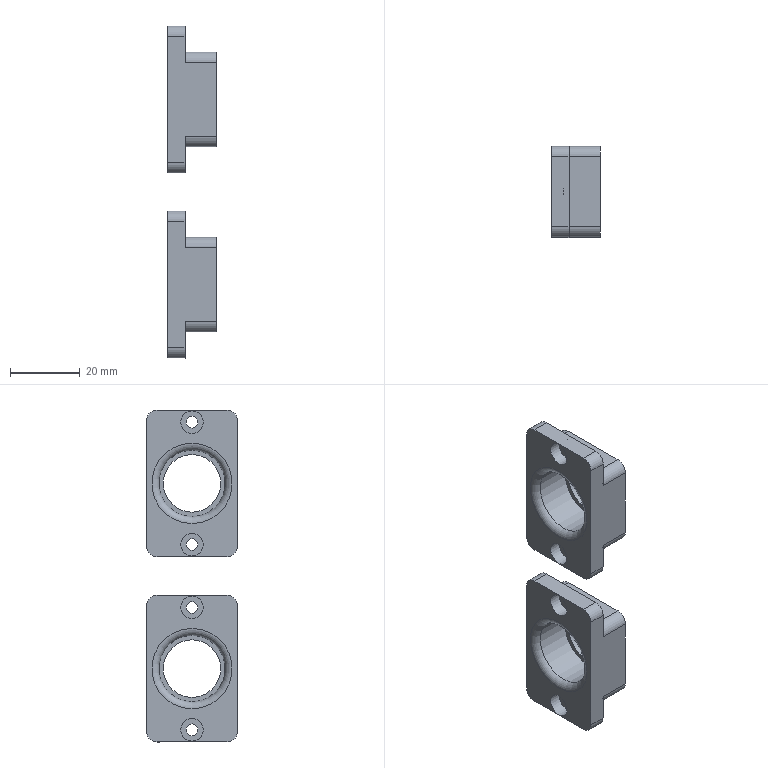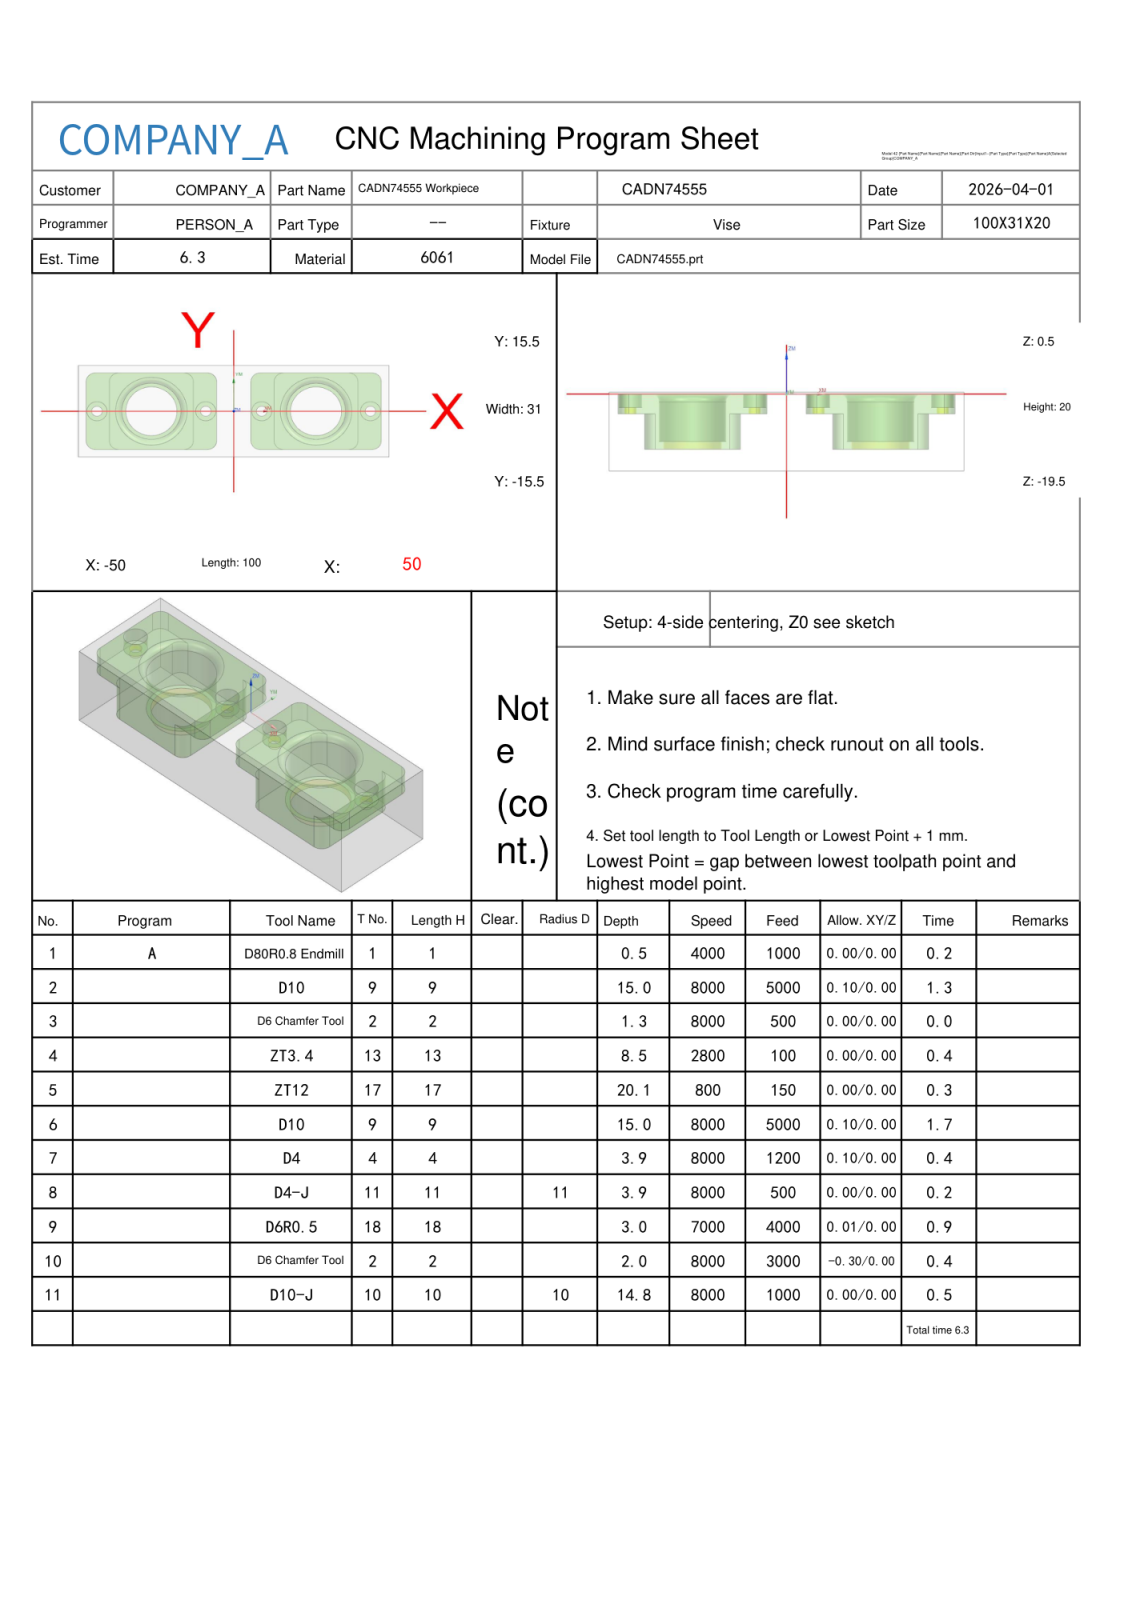NC program | NX | posted by the shop | part box 14 x 26 x 95 mm
Lines 1 to 426 of 19918:
%
O0001
(Machine time: 8.47 MIN)
(===Total Tool:9===)
(T1=D80R0.8 Endmill D=80.  R=0.8  D-  H01 Z=-0.   )
(T9=D10     D=10.  R=0.   D-  H09 Z=-14.5 )
(T2=D6 Chamfer tool   D=6.   R=0.   D-  H02 Z=-1.5  )
(T13=ZT3.4  D=3.4  DR_a=118 D-  H13 Z=-8.02 )
(T17=ZT12   D=12.  DR_a=118 D-  H17 Z=-19.61)
(T4=D4      D=4.   R=0.   D-  H04 Z=-3.4  )
(T11=D4-J   D=4.   R=0.   D11 H11 Z=-3.4  )
(T18=D6R0.5 D=6.   R=0.5  D-  H18 Z=-2.5  )
(T10=D10-J  D=10.  R=0.   D10 H10 Z=-14.3 )
G80 G90 G17 G49 G40
G91 G28 Z0
M01
N1 T01 M06
(D80R0.8 Endmill  D=80. R=0.8 H=01 ce=0.00 di=0.00)
G00 G90 G54 X92.5 Y0.0 M03 S4000
G43 H01 Z20.
M08
Z2.
G01 Z0.0 F1000.
X87.5
X-87.5
X-92.5
Z2.
G00 Z20.
G91 G28 Z0.0
M05
M09
G91 G28 Z0.0
M01
N2 T09 M06
(D10  D=10. R=0. H=09 ce=0.10 di=0.00)
G00 G90 G54 X-26.5 Y18.1 M03 S8000
G43 H09 Z20.
M08
Z.5
G01 X-8.5 Z.413 F5000.
G02 X-.4 Y10. Z.351 I0.0 J-8.1
G01 Y-10. Z.254
G02 X-8.5 Y-18.1 Z.193 I-8.1 J0.0
G01 X-44.5 Z.018
G02 X-52.6 Y-10. Z-.044 I0.0 J8.1
G01 Y10. Z-.141
G02 X-44.5 Y18.1 Z-.202 I8.1 J0.0
G01 X-8.5 Z-.377
G02 X-.4 Y10. Z-.438 I0.0 J-8.1
G01 Y-10. Z-.535
G02 X-8.5 Y-18.1 Z-.597 I-8.1 J0.0
G01 X-44.5 Z-.771
G02 X-52.6 Y-10. Z-.833 I0.0 J8.1
G01 Y10. Z-.93
G02 X-44.5 Y18.1 Z-.992 I8.1 J0.0
G01 X-8.5 Z-1.166
G02 X-.4 Y10. Z-1.228 I0.0 J-8.1
G01 Y-10. Z-1.325
G02 X-8.5 Y-18.1 Z-1.386 I-8.1 J0.0
G01 X-44.5 Z-1.561
G02 X-52.6 Y-10. Z-1.623 I0.0 J8.1
G01 Y10. Z-1.72
G02 X-44.5 Y18.1 Z-1.781 I8.1 J0.0
G01 X-8.5 Z-1.956
G02 X-.4 Y10. Z-2.017 I0.0 J-8.1
G01 Y-10. Z-2.114
G02 X-8.5 Y-18.1 Z-2.176 I-8.1 J0.0
G01 X-44.5 Z-2.35
G02 X-52.6 Y-10. Z-2.412 I0.0 J8.1
G01 Y10. Z-2.509
G02 X-44.5 Y18.1 Z-2.571 I8.1 J0.0
G01 X-8.5 Z-2.745
G02 X-.4 Y10. Z-2.807 I0.0 J-8.1
G01 Y-10. Z-2.904
G02 X-8.5 Y-18.1 Z-2.965 I-8.1 J0.0
G01 X-44.5 Z-3.14
G02 X-52.6 Y-10. Z-3.202 I0.0 J8.1
G01 Y10. Z-3.298
G02 X-44.5 Y18.1 Z-3.36 I8.1 J0.0
G01 X-8.5 Z-3.535
G02 X-.4 Y10. Z-3.596 I0.0 J-8.1
G01 Y-10. Z-3.693
G02 X-8.5 Y-18.1 Z-3.755 I-8.1 J0.0
G01 X-44.5 Z-3.929
G02 X-52.6 Y-10. Z-3.991 I0.0 J8.1
G01 Y10. Z-4.088
G02 X-44.5 Y18.1 Z-4.15 I8.1 J0.0
G01 X-8.5 Z-4.324
G02 X-.4 Y10. Z-4.386 I0.0 J-8.1
G01 Y-10. Z-4.483
G02 X-8.5 Y-18.1 Z-4.544 I-8.1 J0.0
G01 X-44.5 Z-4.719
G02 X-52.6 Y-10. Z-4.78 I0.0 J8.1
G01 Y10. Z-4.877
G02 X-44.5 Y18.1 Z-4.939 I8.1 J0.0
G01 X-8.5 Z-5.114
G02 X-.4 Y10. Z-5.175 I0.0 J-8.1
G01 Y-10. Z-5.272
G02 X-8.5 Y-18.1 Z-5.334 I-8.1 J0.0
G01 X-44.5 Z-5.508
G02 X-52.6 Y-10. Z-5.57 I0.0 J8.1
G01 Y10. Z-5.667
G02 X-44.5 Y18.1 Z-5.729 I8.1 J0.0
G01 X-8.5 Z-5.903
G02 X-.4 Y10. Z-5.965 I0.0 J-8.1
G01 Y-10. Z-6.062
G02 X-8.5 Y-18.1 Z-6.123 I-8.1 J0.0
G01 X-44.5 Z-6.298
G02 X-52.6 Y-10. Z-6.359 I0.0 J8.1
G01 Y10. Z-6.456
G02 X-44.5 Y18.1 Z-6.518 I8.1 J0.0
G01 X-8.5 Z-6.693
G02 X-.4 Y10. Z-6.754 I0.0 J-8.1
G01 Y-10. Z-6.851
G02 X-8.5 Y-18.1 Z-6.913 I-8.1 J0.0
G01 X-44.5 Z-7.087
G02 X-52.6 Y-10. Z-7.149 I0.0 J8.1
G01 Y10. Z-7.246
G02 X-44.5 Y18.1 Z-7.307 I8.1 J0.0
G01 X-8.5 Z-7.482
G02 X-.4 Y10. Z-7.544 I0.0 J-8.1
G01 Y-10. Z-7.641
G02 X-8.5 Y-18.1 Z-7.702 I-8.1 J0.0
G01 X-44.5 Z-7.877
G02 X-52.6 Y-10. Z-7.938 I0.0 J8.1
G01 Y10. Z-8.035
G02 X-44.5 Y18.1 Z-8.097 I8.1 J0.0
G01 X-8.5 Z-8.271
G02 X-.4 Y10. Z-8.333 I0.0 J-8.1
G01 Y-10. Z-8.43
G02 X-8.5 Y-18.1 Z-8.492 I-8.1 J0.0
G01 X-44.5 Z-8.666
G02 X-52.6 Y-10. Z-8.728 I0.0 J8.1
G01 Y10. Z-8.825
G02 X-44.5 Y18.1 Z-8.886 I8.1 J0.0
G01 X-8.5 Z-9.061
G02 X-.4 Y10. Z-9.123 I0.0 J-8.1
G01 Y-10. Z-9.22
G02 X-8.5 Y-18.1 Z-9.281 I-8.1 J0.0
G01 X-44.5 Z-9.456
G02 X-52.6 Y-10. Z-9.517 I0.0 J8.1
G01 Y10. Z-9.614
G02 X-44.5 Y18.1 Z-9.676 I8.1 J0.0
G01 X-8.5 Z-9.85
G02 X-.4 Y10. Z-9.912 I0.0 J-8.1
G01 Y-10. Z-10.009
G02 X-8.5 Y-18.1 Z-10.071 I-8.1 J0.0
G01 X-44.5 Z-10.245
G02 X-52.6 Y-10. Z-10.307 I0.0 J8.1
G01 Y10. Z-10.404
G02 X-44.5 Y18.1 Z-10.465 I8.1 J0.0
G01 X-8.5 Z-10.64
G02 X-.4 Y10. Z-10.702 I0.0 J-8.1
G01 Y-10. Z-10.798
G02 X-8.5 Y-18.1 Z-10.86 I-8.1 J0.0
G01 X-44.5 Z-11.035
G02 X-52.6 Y-10. Z-11.096 I0.0 J8.1
G01 Y10. Z-11.193
G02 X-44.5 Y18.1 Z-11.255 I8.1 J0.0
G01 X-8.5 Z-11.429
G02 X-.4 Y10. Z-11.491 I0.0 J-8.1
G01 Y-10. Z-11.588
G02 X-8.5 Y-18.1 Z-11.65 I-8.1 J0.0
G01 X-44.5 Z-11.824
G02 X-52.6 Y-10. Z-11.886 I0.0 J8.1
G01 Y10. Z-11.983
G02 X-44.5 Y18.1 Z-12.044 I8.1 J0.0
G01 X-8.5 Z-12.219
G02 X-.4 Y10. Z-12.28 I0.0 J-8.1
G01 Y-10. Z-12.377
G02 X-8.5 Y-18.1 Z-12.439 I-8.1 J0.0
G01 X-44.5 Z-12.614
G02 X-52.6 Y-10. Z-12.675 I0.0 J8.1
G01 Y10. Z-12.772
G02 X-44.5 Y18.1 Z-12.834 I8.1 J0.0
G01 X-8.5 Z-13.008
G02 X-.4 Y10. Z-13.07 I0.0 J-8.1
G01 Y-10. Z-13.167
G02 X-8.5 Y-18.1 Z-13.229 I-8.1 J0.0
G01 X-44.5 Z-13.403
G02 X-52.6 Y-10. Z-13.465 I0.0 J8.1
G01 Y10. Z-13.562
G02 X-44.5 Y18.1 Z-13.623 I8.1 J0.0
G01 X-8.5 Z-13.798
G02 X-.4 Y10. Z-13.859 I0.0 J-8.1
G01 Y-10. Z-13.956
G02 X-8.5 Y-18.1 Z-14.018 I-8.1 J0.0
G01 X-44.5 Z-14.193
G02 X-52.6 Y-10. Z-14.254 I0.0 J8.1
G01 Y10. Z-14.351
G02 X-44.5 Y18.1 Z-14.413 I8.1 J0.0
G01 X-26.5 Z-14.5
X-8.5
G02 X-.4 Y10. I0.0 J-8.1
G01 Y-10.
G02 X-8.5 Y-18.1 I-8.1 J0.0
G01 X-44.5
G02 X-52.6 Y-10. I0.0 J8.1
G01 Y10.
G02 X-44.5 Y18.1 I8.1 J0.0
G01 X-26.5
X-26.
Z-13.5
G00 Z20.
X26.5
Z.5
G01 X44.5 Z.413
G02 X52.6 Y10. Z.351 I0.0 J-8.1
G01 Y-10. Z.254
G02 X44.5 Y-18.1 Z.193 I-8.1 J0.0
G01 X8.5 Z.018
G02 X.4 Y-10. Z-.044 I0.0 J8.1
G01 Y10. Z-.141
G02 X8.5 Y18.1 Z-.202 I8.1 J0.0
G01 X44.5 Z-.377
G02 X52.6 Y10. Z-.438 I0.0 J-8.1
G01 Y-10. Z-.535
G02 X44.5 Y-18.1 Z-.597 I-8.1 J0.0
G01 X8.5 Z-.771
G02 X.4 Y-10. Z-.833 I0.0 J8.1
G01 Y10. Z-.93
G02 X8.5 Y18.1 Z-.992 I8.1 J0.0
G01 X44.5 Z-1.166
G02 X52.6 Y10. Z-1.228 I0.0 J-8.1
G01 Y-10. Z-1.325
G02 X44.5 Y-18.1 Z-1.386 I-8.1 J0.0
G01 X8.5 Z-1.561
G02 X.4 Y-10. Z-1.623 I0.0 J8.1
G01 Y10. Z-1.72
G02 X8.5 Y18.1 Z-1.781 I8.1 J0.0
G01 X44.5 Z-1.956
G02 X52.6 Y10. Z-2.017 I0.0 J-8.1
G01 Y-10. Z-2.114
G02 X44.5 Y-18.1 Z-2.176 I-8.1 J0.0
G01 X8.5 Z-2.35
G02 X.4 Y-10. Z-2.412 I0.0 J8.1
G01 Y10. Z-2.509
G02 X8.5 Y18.1 Z-2.571 I8.1 J0.0
G01 X44.5 Z-2.745
G02 X52.6 Y10. Z-2.807 I0.0 J-8.1
G01 Y-10. Z-2.904
G02 X44.5 Y-18.1 Z-2.965 I-8.1 J0.0
G01 X8.5 Z-3.14
G02 X.4 Y-10. Z-3.202 I0.0 J8.1
G01 Y10. Z-3.298
G02 X8.5 Y18.1 Z-3.36 I8.1 J0.0
G01 X44.5 Z-3.535
G02 X52.6 Y10. Z-3.596 I0.0 J-8.1
G01 Y-10. Z-3.693
G02 X44.5 Y-18.1 Z-3.755 I-8.1 J0.0
G01 X8.5 Z-3.929
G02 X.4 Y-10. Z-3.991 I0.0 J8.1
G01 Y10. Z-4.088
G02 X8.5 Y18.1 Z-4.15 I8.1 J0.0
G01 X44.5 Z-4.324
G02 X52.6 Y10. Z-4.386 I0.0 J-8.1
G01 Y-10. Z-4.483
G02 X44.5 Y-18.1 Z-4.544 I-8.1 J0.0
G01 X8.5 Z-4.719
G02 X.4 Y-10. Z-4.78 I0.0 J8.1
G01 Y10. Z-4.877
G02 X8.5 Y18.1 Z-4.939 I8.1 J0.0
G01 X44.5 Z-5.114
G02 X52.6 Y10. Z-5.175 I0.0 J-8.1
G01 Y-10. Z-5.272
G02 X44.5 Y-18.1 Z-5.334 I-8.1 J0.0
G01 X8.5 Z-5.508
G02 X.4 Y-10. Z-5.57 I0.0 J8.1
G01 Y10. Z-5.667
G02 X8.5 Y18.1 Z-5.729 I8.1 J0.0
G01 X44.5 Z-5.903
G02 X52.6 Y10. Z-5.965 I0.0 J-8.1
G01 Y-10. Z-6.062
G02 X44.5 Y-18.1 Z-6.123 I-8.1 J0.0
G01 X8.5 Z-6.298
G02 X.4 Y-10. Z-6.359 I0.0 J8.1
G01 Y10. Z-6.456
G02 X8.5 Y18.1 Z-6.518 I8.1 J0.0
G01 X44.5 Z-6.693
G02 X52.6 Y10. Z-6.754 I0.0 J-8.1
G01 Y-10. Z-6.851
G02 X44.5 Y-18.1 Z-6.913 I-8.1 J0.0
G01 X8.5 Z-7.087
G02 X.4 Y-10. Z-7.149 I0.0 J8.1
G01 Y10. Z-7.246
G02 X8.5 Y18.1 Z-7.307 I8.1 J0.0
G01 X44.5 Z-7.482
G02 X52.6 Y10. Z-7.544 I0.0 J-8.1
G01 Y-10. Z-7.641
G02 X44.5 Y-18.1 Z-7.702 I-8.1 J0.0
G01 X8.5 Z-7.877
G02 X.4 Y-10. Z-7.938 I0.0 J8.1
G01 Y10. Z-8.035
G02 X8.5 Y18.1 Z-8.097 I8.1 J0.0
G01 X44.5 Z-8.271
G02 X52.6 Y10. Z-8.333 I0.0 J-8.1
G01 Y-10. Z-8.43
G02 X44.5 Y-18.1 Z-8.492 I-8.1 J0.0
G01 X8.5 Z-8.666
G02 X.4 Y-10. Z-8.728 I0.0 J8.1
G01 Y10. Z-8.825
G02 X8.5 Y18.1 Z-8.886 I8.1 J0.0
G01 X44.5 Z-9.061
G02 X52.6 Y10. Z-9.123 I0.0 J-8.1
G01 Y-10. Z-9.22
G02 X44.5 Y-18.1 Z-9.281 I-8.1 J0.0
G01 X8.5 Z-9.456
G02 X.4 Y-10. Z-9.517 I0.0 J8.1
G01 Y10. Z-9.614
G02 X8.5 Y18.1 Z-9.676 I8.1 J0.0
G01 X44.5 Z-9.85
G02 X52.6 Y10. Z-9.912 I0.0 J-8.1
G01 Y-10. Z-10.009
G02 X44.5 Y-18.1 Z-10.071 I-8.1 J0.0
G01 X8.5 Z-10.245
G02 X.4 Y-10. Z-10.307 I0.0 J8.1
G01 Y10. Z-10.404
G02 X8.5 Y18.1 Z-10.465 I8.1 J0.0
G01 X44.5 Z-10.64
G02 X52.6 Y10. Z-10.702 I0.0 J-8.1
G01 Y-10. Z-10.798
G02 X44.5 Y-18.1 Z-10.86 I-8.1 J0.0
G01 X8.5 Z-11.035
G02 X.4 Y-10. Z-11.096 I0.0 J8.1
G01 Y10. Z-11.193
G02 X8.5 Y18.1 Z-11.255 I8.1 J0.0
G01 X44.5 Z-11.429
G02 X52.6 Y10. Z-11.491 I0.0 J-8.1
G01 Y-10. Z-11.588
G02 X44.5 Y-18.1 Z-11.65 I-8.1 J0.0
G01 X8.5 Z-11.824
G02 X.4 Y-10. Z-11.886 I0.0 J8.1
G01 Y10. Z-11.983
G02 X8.5 Y18.1 Z-12.044 I8.1 J0.0
G01 X44.5 Z-12.219
G02 X52.6 Y10. Z-12.28 I0.0 J-8.1
G01 Y-10. Z-12.377
G02 X44.5 Y-18.1 Z-12.439 I-8.1 J0.0
G01 X8.5 Z-12.614
G02 X.4 Y-10. Z-12.675 I0.0 J8.1
G01 Y10. Z-12.772
G02 X8.5 Y18.1 Z-12.834 I8.1 J0.0
G01 X44.5 Z-13.008
G02 X52.6 Y10. Z-13.07 I0.0 J-8.1
G01 Y-10. Z-13.167
G02 X44.5 Y-18.1 Z-13.229 I-8.1 J0.0
G01 X8.5 Z-13.403
G02 X.4 Y-10. Z-13.465 I0.0 J8.1
G01 Y10. Z-13.562
G02 X8.5 Y18.1 Z-13.623 I8.1 J0.0
G01 X44.5 Z-13.798
G02 X52.6 Y10. Z-13.859 I0.0 J-8.1
G01 Y-10. Z-13.956
G02 X44.5 Y-18.1 Z-14.018 I-8.1 J0.0
G01 X8.5 Z-14.193
G02 X.4 Y-10. Z-14.254 I0.0 J8.1
G01 Y10. Z-14.351
G02 X8.5 Y18.1 Z-14.413 I8.1 J0.0
G01 X26.5 Z-14.5
X44.5
G02 X52.6 Y10. I0.0 J-8.1
G01 Y-10.
G02 X44.5 Y-18.1 I-8.1 J0.0
G01 X8.5
G02 X.4 Y-10. I0.0 J8.1
G01 Y10.
G02 X8.5 Y18.1 I8.1 J0.0
G01 X26.5
X27.
Z-13.5
G00 Z20.
G91 G28 Z0.0
M05
M09
G91 G28 Z0.0
M01
N3 T02 M06
(D6 Chamfer tool  D=6. R=0. H=02 ce=0.00 di=0.00)
G00 G90 G54 X-44. Y0.0 M03 S8000
G43 H02 Z20.
M08
G98 G81 X-44. Y0.0 Z-.8 R1. F500.
X-26.5
X-9.
X9.
X26.5
X44.
G80
G00 Z20.
G91 G28 Z0.0
M05
M09
G91 G28 Z0.0
M01
N4 T13 M06
(ZT3.4 D=3.4 DR_a=118 H=13)
G00 G90 G54 X-44. Y0.0 M03 S2800
G43 H13 Z20.
M08
G98 G83 X-44. Y0.0 Z-8.021 R1. F100. Q2.
X-9.
X9.
X44.
G80
G00 Z20.
G91 G28 Z0.0
M05
M09
G91 G28 Z0.0
M01
N5 T17 M06
(ZT12 D=12. DR_a=118 H=17)
G00 G90 G54 X-26.5 Y0.0 M03 S800
G43 H17 Z20.
M08
G98 G83 X-26.5 Y0.0 Z-19.605 R1. F150. Q2.
X26.5
G80
G00 Z20.
G91 G28 Z0.0
M05
M09
G91 G28 Z0.0
M01